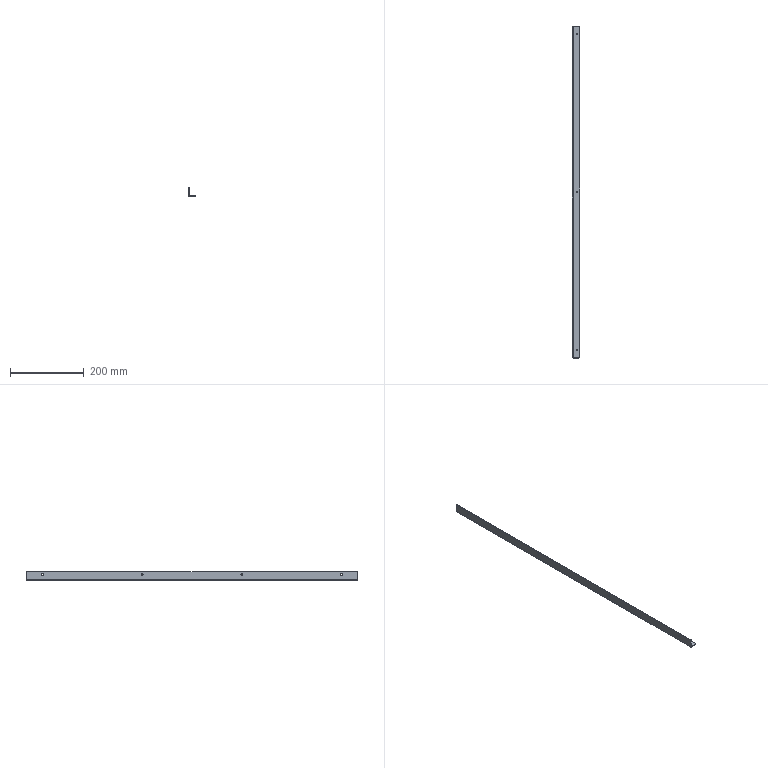Part | STEP file | 1 solid | 32 faces | box 20 x 900 x 23.6 mm | volume 73815 mm3 | cylinder 20 | plane 12 | commonest cylinder face diameters 5 x8 3.3 x6 4 x4 0.2 x1 4.2 x1